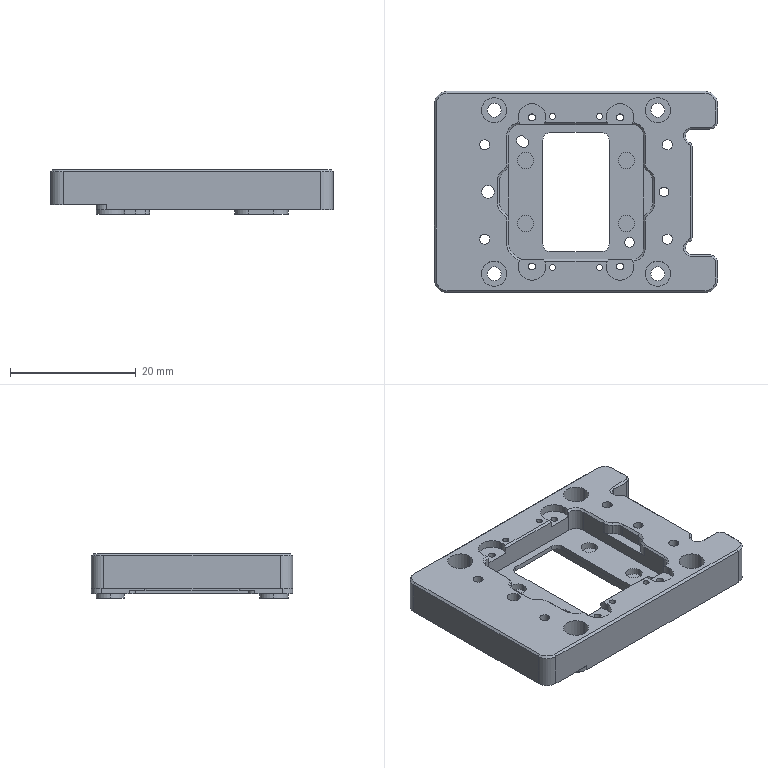NC program | NX | posted with a generic post | part box 45 x 32 x 7.05 mm
Lines 1 to 1283 of 5787:
N10 G17 G21 G94 G90
(FLOOR_WALL , TOOL : D63)
N12 T03 M6
N14 G54
N16 G17 G0 G90 X-60. Y0. S6500 M3
N18 G43 Z30. H3
N20 Z3.
N22 G94 G1 Z0. F1250.
N24 X-57.
N26 X57.
N28 X60.
N30 Z3.
N32 G0 Z30.
N34 M5
(DRILLING , TOOL : D6A45)
N36 T01 M6
N38 G54
N40 G17 G0 G90 X13. Y-13. S5000 M3
N42 G43 Z30. H1
N44 G94 G81 G98 Z-0.6 F250. R3.
N46 X14.5 Y-7.5
N48 X14. Y0.
N50 X14.5 Y7.5
N52 X13. Y13.
N54 X3.75 Y12.
N56 X7. Y11.85
N58 X8. Y5.
N60 Y-5.
N62 X8.5 Y-8.
N64 X7. Y-11.85
N66 X3.75 Y-12.
N68 X-3.75
N70 X-7. Y-11.85
N72 X-13. Y-13.
N74 X-14.5 Y-7.5
N76 X-14. Y0.
N78 X-14.5 Y7.5
N80 X-13. Y13.
N82 X-3.75 Y12.
N84 X-7. Y11.85
N86 X-8.682 Y8.171
N88 X-8. Y5.
N90 Y-5.
N92 G80
N94 G0 X-8. Y-5. Z30.
N96 M5
(DRILLING_COPY , TOOL : 1.6ZT)
N98 T11 M6
N100 G54
N102 G17 G0 G90 X-14.5 Y-7.5 S2000 M3
N104 G43 Z30. H11
N106 G94 G83 G98 Z-7.831 F100. Q1. R3.
N108 Y7.5
N110 X14.5
N112 Y-7.5
N114 G80
N116 G0 X14.5 Y-7.5 Z30.
N118 M5
(DRILLING_COPY_COPY_1 , TOOL : 1.55ZT)
N120 T20 M6
N122 G54
N124 G17 G0 G90 X14. Y0. S2000 M3
N126 G43 Z30. H20
N128 G94 G83 G98 Z-7.816 F100. Q1. R3.
N130 G80
N132 G0 X14. Y0. Z30.
N134 M5
(DRILLING_COPY_COPY , TOOL : 2.2ZT)
N136 T12 M6
N138 G54
N140 G17 G0 G90 X-13. Y13. S1447 M3
N142 G43 Z30. H12
N144 G94 G83 G98 Z-9.211 F100. Q2. R3.
N146 X13.
N148 X-13. Y-13.
N150 X13.
N152 G80
N154 G0 X13. Y-13. Z30.
N156 M5
(DRILLING_COPY_COPY_1_COPY , TOOL : 1.1ZT)
N158 T13 M6
N160 G54
N162 G17 G0 G90 X-7. Y11.85 S2000 M3
N164 G43 Z30. H13
N166 G94 G83 G98 Z-8.88 F100. Q1. R3.
N168 X7. Z-8.18
N170 Y-11.85 Z-8.88
N172 X-7. Z-8.18
N174 G80
N176 G0 X-7. Y-11.85 Z30.
N178 M5
(DRILLING_COPY_COPY_1_COPY_COPY , TOOL : 0.95ZT)
N180 T08 M6
N182 G54
N184 G17 G0 G90 X-3.75 Y-12. S2000 M3
N186 G43 Z30. H8
N188 G94 G83 G98 Z-6.385 F100. Q1. R3.
N190 X3.75
N192 Y12.
N194 X-3.75
N196 G80
N198 G0 X-3.75 Y12. Z30.
N200 M5
(DRILLING_COPY_COPY_COPY , TOOL : 2.05ZT)
N202 T09 M6
N204 G54
N206 G17 G0 G90 X-14. Y0. S1447 M3
N208 G43 Z30. H9
N210 G94 G83 G98 Z-7.966 F100. Q2. R3.
N212 G80
N214 G0 X-14. Y0. Z30.
N216 M5
(ADAPTIVE_MILLING , TOOL : D6)
N218 T06 M6
N220 G54
N222 G17 G0 G90 X-30.144 Y0.013 S9500 M3
N224 G43 Z30. H6
N226 Z-6.05
N228 G94 G1 Z-7.05 F1000.
N230 X-29.181 Y-0.309 F3000.
N232 G3 X-28.537 Y0.013 R0.611
N234 X-28.017 Y2.598 R6.628
N236 X-27.907 Y10.397 R180.736
N238 G2 X-27.877 Y17.595 R582.127
N240 X-25.501 Y20.398 R3.935
N242 X-20.894 Y21.302 R12.338
N244 X-6.645 Y21.392 R469.492
N246 G1 X23.73
N248 X23.805 Y21.391
N250 X23.88 Y21.387
N252 X23.955 Y21.381
N254 X24.029 Y21.372
N256 G2 X26.83 Y19.101 R3.89
N258 X27.783 Y14.658 R11.526
N260 X27.892 Y5.96 R211.965
N262 G1 X27.893 Y-10.84
N264 Y-17.215
N266 X27.892 Y-17.29
N268 X27.888 Y-17.365
N270 X27.882 Y-17.44
N272 X27.874 Y-17.514
N274 G2 X25.548 Y-20.356 R3.894
N276 X21.1 Y-21.289 R11.787
N278 X12.326 Y-21.392 R236.71
N280 G1 X-7.774
N282 X-23.749
N284 X-23.824 Y-21.39
N286 X-23.898 Y-21.385
N288 X-23.973 Y-21.378
N290 X-24.048 Y-21.369
N292 G2 X-26.837 Y-19.085 R3.894
N294 X-27.791 Y-14.566 R11.72
N296 X-27.862 Y-1.518 R292.418
N298 G3 X-27.319 Y9.034 R76.109
N300 G1 X-27.315 Y10.909
N302 X-27.313 Y14.509
N304 X-27.312 Y15.334
N306 X-27.31 Y15.484
N308 X-27.304 Y15.634
N310 X-27.299 Y15.709
N312 X-27.293 Y15.783
N314 X-27.285 Y15.858
N316 G2 X-24.388 Y19.606 R4.858
N318 X-19.582 Y20.651 R12.957
N320 X-10.059 Y20.785 R192.646
N322 G1 X0.441 Y20.786
N324 X21.891
N326 X21.966 Y20.785
N328 X22.116 Y20.779
N330 X22.266 Y20.768
N332 X22.34 Y20.761
N334 G2 X26.128 Y17.807 R4.868
N336 X27.158 Y12.92 R13.32
N338 X27.286 Y2.872 R220.339
N340 G1 X27.287 Y-15.353
N342 X27.286 Y-15.428
N344 X27.281 Y-15.578
N346 X27.277 Y-15.653
N348 X27.265 Y-15.802
N350 G2 X24.342 Y-19.612 R4.852
N352 X19.609 Y-20.648 R12.909
N354 X10.461 Y-20.785 R179.38
N356 G1 X3.186 Y-20.786
N358 X-21.864
N360 X-21.939 Y-20.785
N362 X-22.089 Y-20.78
N364 X-22.164 Y-20.776
N366 X-22.238 Y-20.77
N368 G2 X-26.05 Y-17.965 R4.808
N370 X-27.133 Y-13.321 R12.38
N372 X-27.224 Y-1.925 R144.317
N374 G3 X-26.723 Y11.259 R125.514
N376 G2 X-26.639 Y14.855 R31.892
N378 X-23.197 Y19.001 R5.585
N380 X-17.781 Y20.06 R15.398
N382 X-3.983 Y20.179 R359.36
N384 G1 X20.242 Y20.18
N386 X20.467 Y20.177
N388 X20.617 Y20.173
N390 X20.767 Y20.166
N392 X20.917 Y20.155
N394 G2 X25.375 Y16.923 R5.45
N396 X26.519 Y11.833 R13.725
N398 X26.68 Y0.136 R210.087
N400 X26.65 Y-14.488 R846.011
N402 X23.36 Y-18.908 R5.483
N404 X18.263 Y-20.029 R13.969
N406 X6.941 Y-20.179 R219.596
N408 G1 X-20.284 Y-20.18
N410 X-20.434 Y-20.178
N412 X-20.584 Y-20.173
N414 X-20.734 Y-20.167
N416 X-20.884 Y-20.158
N418 G2 X-25.395 Y-16.886 R5.465
N420 X-26.524 Y-11.792 R13.908
N422 X-26.331 Y1.845 R95.989
N424 G3 X-26.106 Y13.016 R282.676
N426 G2 X-25.261 Y15.849 R5.931
N428 G1 X-24.976 Y16.536
N430 X-24.935 Y16.608
N432 G2 X-21.872 Y18.959 R5.526
N434 X-12.437 Y19.556 R60.192
N436 G1 X-11.162 Y19.563
N438 X-9.587 Y19.568
N440 X-6.962 Y19.572
N442 X0.163 Y19.573
N444 X18.913
N446 X19.138 Y19.57
N448 G2 X22.118 Y18.856 R6.157
N450 X24.167 Y17.608 R5.477
N452 X25.48 Y15.291 R5.884
N454 X26.057 Y5.712 R64.333
N456 X26.042 Y-13.263 R971.054
N458 X25.356 Y-15.62 R5.962
N460 X24.108 Y-17.667 R5.475
N462 X21.791 Y-18.98 R5.884
N464 X12.812 Y-19.552 R60.138
N466 G1 X11.612 Y-19.561
N468 X10.262 Y-19.567
N470 X8.162 Y-19.571
N472 X4.037 Y-19.573
N474 X-18.913
N476 X-19.138 Y-19.57
N478 G2 X-22.102 Y-18.863 R6.151
N480 X-24.167 Y-17.608 R5.5
N482 X-25.48 Y-15.291 R5.884
N484 X-26.057 Y-4.811 R68.436
N486 X-25.65 Y3.933 R579.316
N488 G1 Y13.979
N490 X-25.647 Y14.021
N492 X-25.48 Y15.291
N494 X-25.459 Y15.372
N496 X-25.258 Y15.857
N498 X-25.104 Y16.236
N500 X-24.935 Y16.608
N502 X-24.531 Y17.145
N504 X-24.108 Y17.667
N506 X-23.58 Y18.081
N508 X-23.036 Y18.476
N510 X-22.418 Y18.739
N512 X-21.791 Y18.98
N514 X-20.521 Y19.147
N516 X-20.479 Y19.15
N518 X20.479
N520 X20.521 Y19.147
N522 X21.791 Y18.98
N524 X21.872 Y18.959
N526 X22.149 Y18.844
N528 X22.632 Y18.648
N530 X23.108 Y18.435
N532 X23.645 Y18.031
N534 X24.167 Y17.608
N536 X24.581 Y17.08
N538 X24.976 Y16.536
N540 X25.239 Y15.918
N542 X25.48 Y15.291
N544 X25.647 Y14.021
N546 G2 X25.506 Y9.626 R31.752
N548 G3 X25.475 Y-7.999 R986.646
N550 X25.65 Y-11.235 R14.601
N552 G1 Y-13.979
N554 X25.647 Y-14.021
N556 X25.48 Y-15.291
N558 X25.459 Y-15.372
N560 X25.344 Y-15.649
N562 G3 X26.613 Y-15.908 R-0.66
N564 G1 X26.673 Y-10.299
N566 X26.685 Y-9.099 Z-6.95
N568 X26.882 Y9.539
N570 X26.893 Y10.119 Z-6.998
N572 X26.882 Y10.699 Z-7.047
N574 X26.876 Y10.738 Z-7.05
N576 G3 X25.579 Y10.673 R0.66
N578 G2 X25.263 Y9.468 R4.401
N580 G3 X24.902 Y4.991 R21.417
N582 X24.901 Y-8.806 R734.54
N584 G2 X25.493 Y-10.102 R12.879
N586 G3 X26.492 Y-10.382 R0.662
N588 X26.762 Y-9.73 Z-6.988 R0.714
N590 G1 X26.759 Y-9.269 Z-6.95
N592 X26.651 Y8.966
N594 X26.653 Y9.344 Z-6.982
N596 X26.628 Y9.722 Z-7.013
N598 G3 X26.397 Y10.089 Z-7.05 R0.681
N600 X25.378 Y9.824 R0.662
N602 X24.398 Y5.67 R9.407
N604 X24.314 Y-7.902 R264.987
N606 X24.447 Y-8.296 R2.309
N608 G1 X24.995 Y-9.01
N610 G3 X25.841 Y-9.185 R0.664
N612 X26.179 Y-8.5 Z-6.983 R0.702
N614 G1 X26.181 Y-8.109 Z-6.95
N616 X26.25 Y8.181
N618 X26.254 Y8.514 Z-6.978
N620 X26.235 Y8.846 Z-7.006
N622 G3 X25.934 Y9.269 Z-7.05 R0.668
N624 X25.069 Y9.106 R0.664
N626 X24.024 Y6.498 R4.897
N628 X23.705 Y0.287 R46.885
N630 X23.734 Y-7.137 R135.875
N632 X24.237 Y-8.082 R1.07
N634 G1 X24.42 Y-8.265
N636 X24.447 Y-8.296
N638 G3 X25.255 Y-8.443 R0.665
N640 X25.606 Y-7.765 Z-6.983 R0.702
N642 G1 X25.615 Y-7.374 Z-6.95
N644 X25.966 Y7.805
N646 X25.976 Y8.14 Z-6.978
N648 X25.964 Y8.475 Z-7.006
N650 G3 X25.676 Y8.902 Z-7.05 R0.669
N652 X24.795 Y8.749 R0.664
N654 X23.442 Y5.545 R5.61
N656 X23.104 Y-1.942 R58.845
N658 X23.189 Y-6.737 R41.313
N660 X23.504 Y-7.532 R1.423
N662 G1 X24.046 Y-7.935
N664 G3 X24.782 Y-7.971 R0.666
N666 X25.103 Y-7.317 Z-6.986 R0.705
N668 G1 X25.116 Y-6.883 Z-6.95
N670 X25.53 Y7.243
N672 X25.543 Y7.582 Z-6.978
N674 X25.533 Y7.92 Z-7.007
N676 G3 X25.256 Y8.345 Z-7.05 R0.669
N678 X24.42 Y8.265 R0.664
N680 X23.087 Y5.889 R4.03
N682 X22.546 Y-0.15 R29.605
N684 X22.589 Y-5.997 R56.614
N686 X22.978 Y-7.19 R2.15
N688 G1 X23.035 Y-7.238
N690 X23.097 Y-7.279
N692 X23.16 Y-7.313
N694 X23.213 Y-7.332
N696 X23.294 Y-7.376
N698 X23.534 Y-7.555
N700 G3 X24.263 Y-7.594 R0.666
N702 X24.593 Y-6.945 Z-6.986 R0.705
N704 G1 X24.611 Y-6.512 Z-6.95
N706 X25.172 Y6.896
N708 X25.191 Y7.253 Z-6.98
N710 X25.18 Y7.61 Z-7.01
N712 G3 X24.927 Y8.009 Z-7.05 R0.673
N714 X24.142 Y8.007 R0.665
N716 X22.67 Y5.819 R3.608
N718 X22.003 Y0.626 R21.542
N720 X22.011 Y-5.445 R50.698
N722 X22.558 Y-7.05 R2.776
N724 X23.201 Y-7.328 R4.959
N726 X23.803 Y-7.25 R0.672
N728 X24.093 Y-6.621 Z-6.99 R0.719
N730 G1 X24.116 Y-6.146 Z-6.95
N732 X24.747 Y6.579
N734 X24.769 Y6.935 Z-6.98
N736 X24.76 Y7.292 Z-7.01
N738 G3 X24.509 Y7.693 Z-7.05 R0.673
N740 X23.72 Y7.693 R0.665
N742 X22.14 Y5.393 R3.832
N744 X21.65 Y3.012 R17.062
N746 X21.679 Y-5.687 R384.037
N748 X22.163 Y-6.917 R1.951
N750 G1 X22.225 Y-6.96
N752 X22.291 Y-6.996
N754 X22.714 Y-7.15
N756 G3 X23.526 Y-6.226 R0.661
N758 G1 X22.842 Y-4.922
N760 G3 X21.65 Y-5.313 R0.66
N762 X21.723 Y-6.54 R4.354
N764 X22.328 Y-7.009 R0.932
N766 X23.027 Y-5.929 R0.66
N768 G1 X22.835 Y-5.727
N770 X22.617 Y-5.554
N772 G3 X21.65 Y-6.138 R0.661
N774 X21.746 Y-6.58 R2.208
N776 X22.978 Y-6.321 R0.66
N778 G1 X23.031 Y-5.783
N780 X23.148 Y-4.589 Z-6.95
N782 X24.209 Y6.17
N784 X24.249 Y6.529 Z-6.98
N786 X24.258 Y6.889 Z-7.01
N788 G3 X24.034 Y7.298 Z-7.05 R0.674
N790 X23.294 Y7.376 R0.666
N792 X21.923 Y5.83 R2.8
N794 G1 X21.862 Y5.693
N796 X21.832 Y5.625
N798 X21.776 Y5.486
N800 X21.722 Y5.346
N802 X21.697 Y5.275
N804 X21.673 Y5.204
N806 X21.657 Y5.131
N808 X21.65 Y5.082
N810 Y2.982
N812 G3 X22.945 Y2.8 R0.66
N814 G1 X24.024 Y6.606
N816 G3 X23.143 Y7.306 R0.661
N818 X21.65 Y5.86 R2.144
N820 G1 Y5.035
N822 G3 X22.909 Y4.757 R0.66
N824 G1 X23.651 Y6.377
N826 G3 X22.79 Y7.178 R0.661
N828 X21.678 Y6.37 R1.576
N830 G1 X21.662 Y6.31
N832 X21.65 Y6.239
N834 Y5.789
N836 G3 X22.888 Y5.47 R0.66
N838 G1 X23.285 Y6.207
N840 G3 X22.438 Y7.049 R0.661
N842 X21.661 Y6.305 R0.915
N844 X21.913 Y5.709 R0.608
N846 G1 X22.153 Y5.544
N848 X23.142 Y4.864 Z-6.95
N850 X23.34 Y4.727
N852 X23.504 Y4.551
N854 X23.571 Y4.396
N856 X26.679 Y-7.193
N858 G2 X27.585 Y-12.352 R36.913
N860 X27.514 Y-14.212 R9.083
N862 G1 X27.249 Y-15.968
N864 G2 X26.238 Y-18.01 R4.668
N866 X24.779 Y-19.411 R8.489
N868 X22.342 Y-21.105 R32.788
N870 X21.529 Y-20.748 R0.602
N872 G1 X21.465 Y-20.558
N874 X21.283 Y-20.005 Z-6.999
N876 X21.085 Y-19.458 Z-7.047
N878 X21.068 Y-19.427 Z-7.05
N880 G3 X20.521 Y-19.147 R0.609
N882 G1 X20.479 Y-19.15
N884 X-20.479
N886 X-20.521 Y-19.147
N888 X-21.791 Y-18.98
N890 X-21.872 Y-18.959
N892 X-22.149 Y-18.844
N894 X-22.632 Y-18.648
N896 X-23.108 Y-18.435
N898 X-23.645 Y-18.031
N900 X-24.167 Y-17.608
N902 X-24.581 Y-17.08
N904 X-24.976 Y-16.536
N906 X-25.239 Y-15.918
N908 X-25.48 Y-15.291
N910 X-25.647 Y-14.021
N912 X-25.65 Y-13.979
N914 Y3.946
N916 G3 X-26.162 Y4.545 R0.61
N918 G1 X-27.089 Y4.69
N920 Z-4.05
N922 G0 Z30.
N924 X1.995 Y-4.659
N926 Z1.
N928 G3 X1.995 Y-4.659 Z0.821 I-1.996 J0.409 F1000.
N930 X1.995 Y-4.659 Z0.642 I-1.996 J0.409
N932 X1.995 Y-4.659 Z0.464 I-1.996 J0.409
N934 X1.995 Y-4.659 Z0.285 I-1.996 J0.409
N936 X1.995 Y-4.659 Z0.106 I-1.996 J0.409
N938 X1.995 Y-4.659 Z-0.073 I-1.996 J0.409
N940 X1.995 Y-4.659 Z-0.251 I-1.996 J0.409
N942 X1.995 Y-4.659 Z-0.43 I-1.996 J0.409
N944 X1.995 Y-4.659 Z-0.609 I-1.996 J0.409
N946 X1.995 Y-4.659 Z-0.788 I-1.996 J0.409
N948 X1.995 Y-4.659 Z-0.966 I-1.996 J0.409
N950 X1.995 Y-4.659 Z-1.145 I-1.996 J0.409
N952 X1.995 Y-4.659 Z-1.324 I-1.996 J0.409
N954 X1.995 Y-4.659 Z-1.503 I-1.996 J0.409
N956 X1.995 Y-4.659 Z-1.681 I-1.996 J0.409
N958 X1.995 Y-4.659 Z-1.86 I-1.996 J0.409
N960 X1.995 Y-4.659 Z-2.039 I-1.996 J0.409
N962 X1.995 Y-4.659 Z-2.218 I-1.996 J0.409
N964 X1.995 Y-4.659 Z-2.396 I-1.996 J0.409
N966 X1.995 Y-4.659 Z-2.575 I-1.996 J0.409
N968 X1.995 Y-4.659 Z-2.754 I-1.996 J0.409
N970 X1.995 Y-4.659 Z-2.933 I-1.996 J0.409
N972 X1.995 Y-4.659 Z-3.112 I-1.996 J0.409
N974 X1.995 Y-4.659 Z-3.29 I-1.996 J0.409
N976 X1.995 Y-4.659 Z-3.469 I-1.996 J0.409
N978 X1.995 Y-4.659 Z-3.648 I-1.996 J0.409
N980 X1.995 Y-4.659 Z-3.827 I-1.996 J0.409
N982 X1.995 Y-4.659 Z-4.005 I-1.996 J0.409
N984 X1.995 Y-4.659 Z-4.184 I-1.996 J0.409
N986 X1.995 Y-4.659 Z-4.363 I-1.996 J0.409
N988 X1.995 Y-4.659 Z-4.542 I-1.996 J0.409
N990 X1.995 Y-4.659 Z-4.72 I-1.996 J0.409
N992 X1.995 Y-4.659 Z-4.899 I-1.996 J0.409
N994 X1.995 Y-4.659 Z-5.078 I-1.996 J0.409
N996 X1.995 Y-4.659 Z-5.257 I-1.996 J0.409
N998 X1.995 Y-4.659 Z-5.435 I-1.996 J0.409
N1000 X1.995 Y-4.659 Z-5.614 I-1.996 J0.409
N1002 X1.995 Y-4.659 Z-5.793 I-1.996 J0.409
N1004 X1.995 Y-4.659 Z-5.972 I-1.996 J0.409
N1006 X1.995 Y-4.659 Z-6.15 I-1.996 J0.409
N1008 X1.995 Y-4.659 Z-6.329 I-1.996 J0.409
N1010 X1.995 Y-4.659 Z-6.508 I-1.996 J0.409
N1012 X1.995 Y-4.659 Z-6.687 I-1.996 J0.409
N1014 X1.995 Y-4.659 Z-6.865 I-1.996 J0.409
N1016 X1.995 Y-4.659 Z-7.044 I-1.996 J0.409
N1018 X2.036 Y-4.25 Z-7.05 R2.038
N1020 G1 X1.998
N1022 G3 X1.991 Y-4.411 R-1.998 F3000.
N1024 X1.872 Y-3.968 R0.835
N1026 X0.697 Y-4.157 R0.661
N1028 G1 X0.619 Y-4.412
N1030 X0.581 Y-4.676
N1032 G3 X1.829 Y-4.946 R0.66
N1034 X2.049 Y-3.516 R1.633
N1036 X-2.1 Y-3.513 R2.175
N1038 X-1.999 Y-5.151 R5.352
N1040 X-0.712 Y-6.35 R1.934
N1042 X0.925 Y-6.241 R5.105
N1044 X2.1 Y-5.02 R1.877
N1046 G1 Y-3.886
N1048 G3 X0.33 Y-1.763 R1.938
N1050 X-2.058 Y-2.833 R2.365
N1052 X-2.1 Y-3.535 R4.622
N1054 X-1.417 Y-4.195 R0.663
N1056 G1 X1.563 Y-4.085
N1058 G3 X2.1 Y-3.436 R0.664
N1060 X0.676 Y-1.574 R1.806
N1062 X-2.03 Y-2.371 R2.477
N1064 X-2.1 Y-3.065 R1.933
N1066 X-1.456 Y-3.725 R0.663
N1068 G1 X1.529 Y-3.79
N1070 G3 X2.1 Y-3.136 R0.664
N1072 X0.798 Y-1.342 R1.752
N1074 X-1.979 Y-1.924 R2.61
N1076 X-2.1 Y-2.634 R1.239
N1078 X-1.486 Y-3.293 R0.663
N1080 G1 X0.007 Y-3.402
N1082 X1.502 Y-3.493
N1084 G3 X2.1 Y-2.836 R0.664
N1086 X0.915 Y-1.112 R1.714
N1088 X-1.957 Y-1.556 R2.647
N1090 X-2.1 Y-2.29 R1.144
N1092 X-1.496 Y-2.947 R0.664
N1094 G1 X-0.003 Y-3.081
N1096 X1.493 Y-3.194
N1098 G3 X2.1 Y-2.536 R0.664
N1100 X0.961 Y-0.856 R1.701
N1102 X-1.929 Y-1.194 R2.676
N1104 X-2.1 Y-1.968 R1.076
N1106 X-1.501 Y-2.625 R0.664
N1108 G1 X-0.007 Y-2.77
N1110 X1.488 Y-2.895
N1112 G3 X2.1 Y-2.236 R0.664
N1114 X1.011 Y-0.597 R1.7
N1116 X-1.944 Y-0.888 R2.636
N1118 X-2.1 Y-1.64 R1.105
N1120 X-1.508 Y-2.297 R0.664
N1122 G1 X1.473 Y-2.596
N1124 G3 X2.1 Y-1.936 R0.663
N1126 X0.995 Y-0.302 R1.726
N1128 X-1.905 Y-0.529 R2.672
N1130 X-2.1 Y-1.321 R1.02
N1132 X-1.529 Y-1.975 R0.664
N1134 G1 X1.453 Y-2.371
N1136 G3 X2.1 Y-1.711 R0.663
N1138 X0.983 Y-0.004 R1.767
N1140 X-1.914 Y-0.227 R2.644
N1142 X-2.1 Y-1.011 R1.037
N1144 X-1.531 Y-1.664 R0.664
N1146 G1 X1.451 Y-2.071
N1148 G3 X2.1 Y-1.411 R0.663
N1150 X1.043 Y0.259 R1.754
N1152 X-1.919 Y0.078 R2.628
N1154 X-2.1 Y-0.702 R1.046
N1156 X-1.533 Y-1.355 R0.664
N1158 G1 X1.45 Y-1.771
N1160 G3 X2.1 Y-1.111 R0.663
N1162 X0.971 Y0.594 R1.797
N1164 X-1.923 Y0.383 R2.603
N1166 X-2.1 Y-0.397 R1.061
N1168 X-1.534 Y-1.05 R0.664
N1170 G1 X1.449 Y-1.471
N1172 G3 X2.1 Y-0.811 R0.663
N1174 X0.967 Y0.894 R1.813
N1176 X-1.926 Y0.687 R2.597
N1178 X-2.1 Y-0.092 R1.072
N1180 X-1.552 Y-0.743 R0.664
N1182 G1 X1.432 Y-1.246
N1184 G3 X2.1 Y-0.586 R0.663
N1186 X0.966 Y1.194 R1.832
N1188 X-1.873 Y1.044 R2.644
N1190 X-2.1 Y0.213 R0.984
N1192 X-1.553 Y-0.437 R0.664
N1194 G1 X1.431 Y-0.946
N1196 G3 X2.1 Y-0.286 R0.663
N1198 X0.964 Y1.494 R1.836
N1200 X-1.873 Y1.349 R2.633
N1202 X-2.1 Y0.518 R0.985
N1204 X-1.554 Y-0.132 R0.664
N1206 G1 X1.43 Y-0.646
N1208 G3 X2.1 Y0.014 R0.663
N1210 X0.896 Y1.828 R1.864
N1212 X-1.927 Y1.601 R2.558
N1214 X-2.1 Y0.823 R1.073
N1216 X-1.555 Y0.173 R0.664
N1218 G1 X1.429 Y-0.346
N1220 G3 X2.1 Y0.314 R0.663
N1222 X0.963 Y2.095 R1.846
N1224 X-1.873 Y1.957 R2.623
N1226 X-2.1 Y1.126 R0.984
N1228 X-1.556 Y0.477 R0.664
N1230 G1 X1.429 Y-0.046
N1232 G3 X2.1 Y0.614 R0.663
N1234 X0.963 Y2.395 R1.846
N1236 X-1.874 Y2.26 R2.631
N1238 X-2.1 Y1.431 R0.985
N1240 X-1.557 Y0.781 R0.664
N1242 G1 X1.428 Y0.254
N1244 G3 X2.1 Y0.914 R0.663
N1246 X0.963 Y2.695 R1.848
N1248 X-1.874 Y2.564 R2.626
N1250 X-2.1 Y1.735 R0.985
N1252 X-1.557 Y1.085 R0.664
N1254 G1 X1.427 Y0.554
N1256 G3 X2.1 Y1.214 R0.663
N1258 X0.963 Y2.996 R1.849
N1260 X-1.874 Y2.867 R2.626
N1262 X-2.1 Y2.038 R0.985
N1264 X-1.558 Y1.389 R0.664
N1266 G1 X1.426 Y0.854
N1268 G3 X2.1 Y1.514 R0.663
N1270 X0.963 Y3.296 R1.85
N1272 X-1.873 Y3.171 R2.624
N1274 X-2.1 Y2.341 R0.984
N1276 X-1.559 Y1.691 R0.664
N1278 G1 X1.426 Y1.154
N1280 G3 X2.1 Y1.814 R0.663
N1282 X0.964 Y3.597 R1.855
N1284 X-1.873 Y3.474 R2.625
N1286 X-2.1 Y2.644 R0.984
N1288 X-1.56 Y1.995 R0.664
N1290 G1 X1.425 Y1.454
N1292 G3 X2.1 Y2.114 R0.663
N1294 X0.964 Y3.897 R1.854
N1296 X-1.873 Y3.776 R2.621
N1298 X-2.1 Y2.945 R0.984
N1300 X-1.56 Y2.296 R0.664
N1302 G1 X1.425 Y1.754
N1304 G3 X2.1 Y2.414 R0.663
N1306 X1.03 Y4.162 R1.831
N1308 X-1.872 Y4.079 R2.63
N1310 X-2.1 Y3.247 R0.983
N1312 X-1.56 Y2.598 R0.664
N1314 G1 X1.424 Y2.054
N1316 G3 X2.1 Y2.714 R0.663
N1318 X0.966 Y4.499 R1.857
N1320 X-1.924 Y4.331 R2.556
N1322 X-2.1 Y3.55 R1.067
N1324 X-1.561 Y2.901 R0.664
N1326 G1 X1.424 Y2.354
N1328 G3 X2.1 Y3.014 R0.663
N1330 X0.968 Y4.8 R1.86
N1332 X-1.869 Y4.686 R2.618
N1334 X-2.1 Y3.854 R0.977
N1336 X-1.562 Y3.205 R0.664
N1338 G1 X1.423 Y2.654
N1340 G3 X2.1 Y3.314 R0.663
N1342 X0.968 Y5.101 R1.862
N1344 X-1.869 Y4.99 R2.619
N1346 X-2.1 Y4.158 R0.976
N1348 X-1.563 Y3.509 R0.664
N1350 G1 X1.422 Y2.954
N1352 G3 X2.1 Y3.614 R0.663
N1354 X0.969 Y5.402 R1.865
N1356 X-1.868 Y5.294 R2.619
N1358 X-2.1 Y4.462 R0.973
N1360 X-1.563 Y3.814 R0.664
N1362 G1 X1.421 Y3.254
N1364 G3 X2.1 Y3.914 R0.663
N1366 X0.97 Y5.702 R1.864
N1368 X-1.866 Y5.596 R2.613
N1370 X-2.1 Y4.765 R0.971
N1372 X-1.564 Y4.117 R0.664
N1374 G1 X1.421 Y3.554
N1376 G3 X2.1 Y4.214 R0.663
N1378 X0.972 Y6.004 R1.872
N1380 X-1.878 Y5.887 R2.615
N1382 X-2.1 Y5.137 R0.895
N1384 X-1.58 Y4.492 R0.664
N1386 G1 X-0.088 Y4.165
N1388 X1.406 Y3.855
N1390 G3 X2.1 Y4.514 R0.663
N1392 X0.773 Y6.35 R1.802
N1394 G1 X-0.202
N1396 G3 X-0.512 Y5.108 R0.66
N1398 G1 X1.225 Y4.19
N1400 G3 X2.1 Y4.814 R0.662
N1402 X1.249 Y6.335 R1.414
N1404 G1 X1.163 Y6.35
N1406 X0.713
N1408 G3 X0.303 Y5.173 R0.661
N1410 G1 X1.118 Y4.538
N1412 G3 X2.1 Y5.114 R0.661
N1414 X1.616 Y6.289 R1.151
N1416 X1.148 Y6.35 R2.349
N1418 X0.694 Y5.211 R0.661
N1420 G1 X1.072 Y4.866
N1422 G3 X2.1 Y5.414 R0.661
N1424 X1.423 Y6.345 R0.78
N1426 G1 X-0.559 Y6.35
N1428 G3 X-1.859 Y6.114 R2.034
N1430 X-2.1 Y5.398 R0.828
N1432 X-0.964 Y4.941 R0.661
N1434 G1 X-0.75 Y5.157
N1436 X-0.566 Y5.4
N1438 G3 X-1.159 Y6.35 R0.661
N1440 X-2.095 Y5.673 R0.782
N1442 X-1.656 Y5.036 R0.604
N1444 G1 X-1.367 Y5.011 Z-7.026
N1446 X-1.076 Z-7.001
N1448 G2 X-0.586 Y4.682 Z-6.95 R0.603
N1450 G1 X-0.544 Y4.551
N1452 X-0.523 Y4.414
N1454 X-0.531 Y-3.524
N1456 X-0.58 Y-3.689
N1458 G2 X-1.232 Y-4.038 Z-7.016 R0.637
N1460 G1 X-1.64 Y-4.055 Z-7.05
N1462 G3 X-2.1 Y-4.638 R0.605
N1464 X-1.252 Y-6.326 R1.591
N1466 G1 X-1.179 Y-6.342
N1468 X-1.125 Y-6.35
N1470 X-0.675
N1472 G3 X-0.267 Y-5.171 R0.661
N1474 G1 X-1.12 Y-4.511
N1476 G3 X-2.1 Y-5.088 R0.661
N1478 X-1.555 Y-6.306 R1.152
N1480 G1 X-1.069 Y-6.35
N1482 G3 X-0.652 Y-5.178 R0.661
N1484 G1 X-1.111 Y-4.816
N1486 G3 X-2.1 Y-5.388 R0.661
N1488 X-1.298 Y-6.35 R0.79
N1490 G1 X0.413
N1492 G3 X2.065 Y-5.559 R1.604
N1494 G1 X2.1 Y-4.951
N1496 G3 X0.945 Y-4.515 R0.661
N1498 G1 X0.229 Y-5.34
N1500 G3 X0.788 Y-6.35 R0.661
N1502 X2.003 Y-5.926 R1.313
N1504 X2.1 Y-5.398 R1.21
N1506 X0.961 Y-4.944 R0.661
N1508 G1 X0.75 Y-5.161
N1510 X0.569 Y-5.404
N1512 G3 X1.163 Y-6.35 R0.661
N1514 X2.1 Y-5.623 R0.78
N1516 X1.625 Y-5.032 R0.611
N1518 G1 X0.589 Y-4.802
N1520 Z-4.05
N1522 G0 Z30.
N1524 X-0.622 Y0.875
N1526 Z-2.699
N1528 G1 Z-3.699 F1000.
N1530 X-1.917 Y0.259 F3000.
N1532 X-2.044 Y0.144
N1534 X-2.138 Y0.
N1536 G3 X-2.658 Y-2.968 R8.162
N1538 X-2.557 Y-5.579 R8.699
N1540 X-1.093 Y-6.696 R1.694
N1542 X1.502 Y-6.713 R5.123
N1544 X2.407 Y-5.427 R1.569
N1546 X2.723 Y-0.87 R25.535
N1548 X2.685 Y5.053 R80.998
N1550 X1.184 Y6.661 R1.659
N1552 X-1.486 Y6.717 R5.369
N1554 X-2.419 Y5.369 R1.612
N1556 X-2.735 Y1.636 R27.994
N1558 X-3.227 Y-4.037 R43.398
N1560 X-2.441 Y-6.318 R3.222
N1562 X1.514 Y-7.027 R4.121
N1564 X2.787 Y-5.26 R2.599
N1566 X3.284 Y-0.724 R19.395
N1568 X3.254 Y4.448 R50.158
N1570 X1.043 Y7.039 R2.731
N1572 X-1.663 Y6.947 R3.641
N1574 X-2.832 Y5.094 R2.852
N1576 X-3.408 Y1.089 R38.498
N1578 X-3.721 Y-4.068 R26.237
N1580 X-0.637 Y-7.528 R3.633
N1582 X1.484 Y-7.35 R4.911
N1584 X3.146 Y-5.322 R3.253
N1586 X3.832 Y-0.74 R16.416
N1588 X3.772 Y4.278 R29.237
N1590 X0.684 Y7.512 R3.707
N1592 X-1.586 Y7.304 R4.474
N1594 X-3.207 Y5.144 R3.484
N1596 X-4.272 Y-3.388 R32.466
N1598 X-2.843 Y-6.825 R4.794
N1600 X-1.635 Y-7.55 R2.909
N1602 G1 X0.536
N1604 G3 X3.136 Y-6.152 R2.543
N1606 X4.264 Y-2.062 R10.109
N1608 X4.337 Y3.85 R27.376
N1610 X1.745 Y7.533 R4.484
N1612 G1 X1.671 Y7.547
N1614 X1.648 Y7.55
N1616 X0.448
N1618 G3 X-0.113 Y7.237 R0.67
N1620 X-0.201 Y6.683 Z-3.651 R0.86
N1622 G1 X-0.167 Y6.057 Z-3.599
N1624 X0.502 Y-6.031
N1626 X0.565 Y-7.027 Z-3.682
N1628 X0.636 Y-7.215 Z-3.699
N1630 G3 X1.211 Y-7.55 R0.67
N1632 X3.26 Y-6.528 R2.269
N1634 X4.695 Y-2.627 R8.503
N1636 X4.828 Y3.872 R21.837
N1638 X2.554 Y7.506 R5.136
N1640 X1.619 Y7.55 R4.681
N1642 X1.058 Y7.237 R0.67
N1644 X0.959 Y6.712 Z-3.654 R0.908
N1646 G1 X0.957 Y6.055 Z-3.599
N1648 X0.928 Y-6.033
N1650 X0.922 Y-6.525 Z-3.64
N1652 X0.94 Y-7.017 Z-3.681
N1654 X1.013 Y-7.218 Z-3.699
N1656 G3 X1.586 Y-7.55 R0.67
N1658 X3.596 Y-6.595 R2.284
N1660 X5.198 Y-2.602 R8.525
N1662 X5.303 Y3.962 R18.519
N1664 X3.275 Y7.453 R5.792
N1666 X2.308 Y7.55 R2.079
N1668 X1.746 Y7.235 R0.67
N1670 X1.643 Y6.679 Z-3.651 R1.033
N1672 G1 X1.627 Y6.054 Z-3.599
N1674 X1.322 Y-6.034
N1676 X1.305 Y-6.521 Z-3.64
N1678 X1.313 Y-7.008 Z-3.68
N1680 X1.388 Y-7.218 Z-3.699
N1682 G3 X1.961 Y-7.55 R0.67
N1684 X4.034 Y-6.555 R2.377
N1686 X5.701 Y-2.587 R8.757
N1688 X5.76 Y4.116 R16.384
N1690 X3.86 Y7.444 R6.01
N1692 X2.952 Y7.55 R1.787
N1694 X2.389 Y7.234 R0.67
N1696 X2.283 Y6.688 Z-3.652 R1.064
N1698 G1 X2.254 Y6.053 Z-3.599
N1700 X1.713 Y-6.035
N1702 X1.686 Y-6.517 Z-3.639
N1704 X1.687 Y-7. Z-3.68
N1706 X1.763 Y-7.218 Z-3.699
N1708 G3 X2.336 Y-7.55 R0.67
N1710 X4.425 Y-6.58 R2.431
N1712 X6.218 Y-2.506 R8.824
N1714 X6.177 Y4.406 R15.006
N1716 X4.443 Y7.417 R6.054
N1718 X3.495 Y7.55 R1.607
N1720 X2.932 Y7.233 R0.67
N1722 X2.824 Y6.691 Z-3.652 R1.093
N1724 G1 X2.791 Y6.052 Z-3.599
N1726 X2.169 Y-6.035
N1728 X2.138 Y-6.516 Z-3.639
N1730 X2.136 Y-6.997 Z-3.679
N1732 X2.214 Y-7.219 Z-3.699
N1734 G3 X2.786 Y-7.55 R0.67
N1736 X4.871 Y-6.558 R2.513
N1738 X6.752 Y-2.362 R9.07
N1740 X6.567 Y4.759 R14.177
N1742 X4.966 Y7.424 R5.703
N1744 X4.023 Y7.55 R1.662
N1746 X3.458 Y7.232 R0.67
N1748 X3.349 Y6.697 Z-3.653 R1.114
N1750 G1 X3.309 Y6.051 Z-3.599
N1752 X2.553 Y-6.036
N1754 X2.517 Y-6.514 Z-3.639
N1756 X2.511 Y-6.993 Z-3.679
N1758 X2.589 Y-7.219 Z-3.699
N1760 G3 X3.161 Y-7.55 R0.67
N1762 X5.268 Y-6.599 R2.552
N1764 X7.268 Y-2.298 R9.078
N1766 G1 X7.55 Y-0.466
N1768 G3 X7.364 Y3.572 R21.543
N1770 X5.67 Y7.271 R7.167
N1772 X5.15 Y7.55 R1.051
N1774 G1 X4.55
N1776 G3 X3.955 Y7.176 R0.669
N1778 X3.999 Y6.51 Z-3.641 R0.717
N1780 G1 X4.211 Y6.053 Z-3.599
N1782 X6.04 Y2.121
N1784 X6.194 Y1.781 Z-3.63
N1786 X6.372 Y1.453 Z-3.661
N1788 G3 X6.745 Y1.215 Z-3.699 R0.678
N1790 X7.55 Y1.859 R0.662
N1792 X7.447 Y4.701 R15.562
N1794 X5.985 Y7.429 R4.871
N1796 X5.125 Y7.55 R1.522
N1798 X4.555 Y6.556 R0.661
N1800 G1 X5.461 Y5.004
N1802 X6.383 Y3.461
N1804 G3 X7.55 Y3.884 R0.661
N1806 X7.292 Y6.175 R5.663
N1808 X6.267 Y7.514 R2.368
N1810 X5.581 Y7.55 R9.137
N1812 X5.039 Y6.513 R0.661
N1814 G1 X6.414 Y4.551
N1816 G3 X7.55 Y5.009 R0.661
N1818 X7.116 Y7.095 R3.318
N1820 X6.095 Y7.55 R0.97
N1822 X5.567 Y6.493 R0.661
N1824 G1 X6.431 Y5.36
N1826 G3 X7.55 Y5.834 R0.661
N1828 X7.143 Y7.379 R2.002
N1830 X6.443 Y7.55 R0.971
N1832 X5.938 Y6.465 R0.661
N1834 G1 X6.46 Y5.858
N1836 G3 X7.55 Y6.359 R0.661
N1838 X7.275 Y7.392 R1.207
N1840 X6.673 Y7.55 R1.039
N1842 X6.503 Y6.252 R0.66
N1844 X7.031 Y6.189 R1.075
N1846 X7.475 Y7.13 R0.662
N1848 X6.823 Y7.55 R0.732
N1850 G1 X-0.497
N1852 G3 X-3.116 Y6.183 R2.556
N1854 X-4.334 Y2.343 R11.441
N1856 X-4.749 Y-3.623 R22.148
N1858 X-2.587 Y-7.482 R5.142
N1860 X-1.598 Y-7.55 R2.875
N1862 X-1.036 Y-7.236 R0.67
N1864 X-0.931 Y-6.682 Z-3.651 R1.04
N1866 G1 X-0.912 Y-6.054 Z-3.599
N1868 X-0.538 Y6.033
N1870 X-0.517 Y6.519 Z-3.64
N1872 X-0.523 Y7.005 Z-3.68
N1874 X-0.599 Y7.218 Z-3.699
N1876 G3 X-1.172 Y7.55 R0.67
N1878 X-3.234 Y6.554 R2.279
N1880 X-4.77 Y2.763 R9.305
N1882 X-5.236 Y-3.64 R19.12
N1884 X-3.231 Y-7.459 R5.67
N1886 X-2.347 Y-7.55 R1.954
N1888 X-1.783 Y-7.234 R0.67
N1890 X-1.675 Y-6.692 Z-3.652 R1.093
N1892 G1 X-1.642 Y-6.053 Z-3.599
N1894 X-1.006 Y6.034
N1896 X-0.975 Y6.515 Z-3.639
N1898 X-0.972 Y6.996 Z-3.679
N1900 X-1.049 Y7.218 Z-3.699
N1902 G3 X-1.622 Y7.55 R0.67
N1904 X-3.619 Y6.563 R2.316
N1906 X-5.323 Y2.603 R9.559
N1908 X-5.699 Y-3.797 R16.831
N1910 X-3.863 Y-7.402 R6.062
N1912 X-2.898 Y-7.55 R1.531
N1914 X-2.334 Y-7.233 R0.67
N1916 X-2.224 Y-6.698 Z-3.653 R1.117
N1918 G1 X-2.182 Y-6.052 Z-3.599
N1920 X-1.391 Y6.035
N1922 X-1.354 Y6.512 Z-3.639
N1924 X-1.346 Y6.991 Z-3.679
N1926 X-1.424 Y7.218 Z-3.699
N1928 G3 X-1.997 Y7.55 R0.67
N1930 X-4.01 Y6.584 R2.391
N1932 X-5.873 Y2.453 R9.603
N1934 X-6.095 Y-4.236 R14.955
N1936 X-4.435 Y-7.37 R6.045
N1938 X-4.028 Y-7.55 R1.403
N1940 G1 X-3.428
N1942 G3 X-2.863 Y-7.232 R0.67
N1944 X-2.751 Y-6.703 Z-3.654 R1.141
N1946 G1 X-2.701 Y-6.052 Z-3.599
N1948 X-1.775 Y6.035
N1950 X-1.733 Y6.51 Z-3.639
N1952 X-1.721 Y6.986 Z-3.679
N1954 X-1.799 Y7.218 Z-3.699
N1956 G3 X-2.372 Y7.55 R0.67
N1958 X-4.456 Y6.561 R2.486
N1960 X-6.403 Y2.388 R9.697
N1962 X-6.474 Y-4.661 R14.037
N1964 X-4.892 Y-7.419 R5.556
N1966 X-4.02 Y-7.55 R1.466
N1968 X-3.455 Y-7.23 R0.67
N1970 G1 X-3.369 Y-6.984 Z-3.677
N1972 X-3.342 Y-6.726 Z-3.656
N1974 X-3.28 Y-6.051 Z-3.599
N1976 X-2.163 Y6.036
N1978 X-2.088 Y6.93 Z-3.674
N1980 X-2.119 Y7.077 Z-3.686
N1982 X-2.174 Y7.217 Z-3.699
N1984 G3 X-2.747 Y7.55 R0.67
N1986 X-4.907 Y6.547 R2.594
N1988 X-6.997 Y2.037 R9.947
N1990 X-6.814 Y-5.146 R13.316
N1992 X-5.349 Y-7.456 R4.822
N1994 X-4.536 Y-7.55 R1.734
N1996 X-3.97 Y-7.229 R0.67
N1998 X-3.851 Y-6.674 Z-3.651 R1.331
N2000 G1 X-3.787 Y-6.05 Z-3.599
N2002 X-2.546 Y6.037
N2004 X-2.463 Y6.925 Z-3.673
N2006 X-2.493 Y7.075 Z-3.686
N2008 X-2.549 Y7.217 Z-3.699
N2010 G3 X-3.122 Y7.55 R0.67
N2012 X-5.36 Y6.543 R2.686
N2014 X-7.55 Y1.828 R9.902
N2016 X-7.521 Y-3.871 R489.075
N2018 X-6.03 Y-7.318 R5.79
N2020 X-5.038 Y-7.55 R1.23
N2022 X-4.456 Y-6.579 R0.661
N2024 G1 X-6.308 Y-3.111
N2026 G3 X-7.55 Y-3.422 R0.66
N2028 X-7.411 Y-5.658 R8.32
N2030 X-6.287 Y-7.472 R3.291
N2032 X-5.5 Y-7.55 R1.965
N2034 X-4.949 Y-6.528 R0.661
N2036 G1 X-6.403 Y-4.326
N2038 G3 X-7.55 Y-4.772 R0.661
N2040 X-7.194 Y-6.883 R3.871
N2042 X-5.968 Y-7.55 R1.088
N2044 X-5.441 Y-6.492 R0.661
N2046 G1 X-6.437 Y-5.192
N2048 G3 X-7.55 Y-5.672 R0.661
N2050 X-7.118 Y-7.363 R2.255
N2052 X-6.409 Y-7.55 R0.935
N2054 X-5.888 Y-6.485 R0.661
N2056 G1 X-6.443 Y-5.786
N2058 G3 X-7.55 Y-6.272 R0.661
N2060 X-7.319 Y-7.339 R1.464
N2062 X-6.673 Y-7.55 R0.872
N2064 X-6.268 Y-6.369 R0.661
N2066 G1 X-6.459 Y-6.22
N2068 X-6.669 Y-6.1
N2070 G3 X-7.55 Y-6.722 R0.662
N2072 X-7.145 Y-7.467 R0.761
N2074 G1 X-6.553 Y-7.367
N2076 G3 X-6.188 Y-7.176 R0.705
N2078 X-5.979 Y-6.687 Z-3.654 R0.912
N2080 G1 X-5.834 Y-6.044 Z-3.599
N2082 X-3.127 Y5.944
N2084 X-3.015 Y6.41 Z-3.639
N2086 X-2.932 Y6.883 Z-3.679
N2088 X-2.973 Y7.118 Z-3.699
N2090 X-3.017 Y7.212
N2092 X-3.076 Y7.298
N2094 X-3.147 Y7.374
N2096 G3 X-4.096 Y7.545 R1.244
N2098 X-6.257 Y6.036 R3.55
N2100 X-7.55 Y3.532 R8.774
N2102 G1 Y1.807
N2104 G3 X-6.847 Y1.148 R0.663
N2106 X-6.262 Y1.578 Z-3.635 R0.706
N2108 G1 X-6.047 Y1.957 Z-3.599
N2110 X-3.749 Y6.03
N2112 X-3.559 Y6.359 Z-3.631
N2114 X-3.391 Y6.7 Z-3.663
N2116 G3 X-3.407 Y7.13 Z-3.699 R0.682
N2118 X-4.022 Y7.55 R0.666
N2120 X-6.274 Y6.558 R2.784
N2122 X-7.549 Y4.638 R5.055
N2124 X-6.439 Y4.155 R0.661
N2126 G1 X-3.951 Y6.485
N2128 G3 X-4.472 Y7.55 R0.661
N2130 X-6.785 Y6.519 R2.858
N2132 X-7.55 Y5.415 R2.56
N2134 G1 Y3.465
N2136 G3 X-6.318 Y3.136 R0.66
N2138 G1 X-5.303 Y4.892
N2140 X-4.304 Y6.657
N2142 G3 X-4.922 Y7.55 R0.662
N2144 X-7.525 Y6.096 R2.805
N2146 G1 X-7.542 Y6.023
N2148 X-7.55 Y6.002
N2150 Y5.402
N2152 G3 X-6.428 Y4.93 R0.661
N2154 G1 X-4.841 Y6.497
N2156 G3 X-5.372 Y7.55 R0.661
N2158 X-7.507 Y6.575 R2.183
N2160 X-7.55 Y5.943 R4.216
N2162 X-6.452 Y5.449 R0.661
N2164 G1 X-5.31 Y6.473
N2166 G3 X-5.822 Y7.55 R0.661
N2168 X-7.513 Y6.914 R1.811
N2170 G1 X-7.521 Y6.893
N2172 X-7.531 Y6.855
N2174 X-7.55 Y6.699
N2176 Y6.324
N2178 G3 X-6.444 Y5.837 R0.661
N2180 G1 X-5.754 Y6.48
N2182 G3 X-6.272 Y7.55 R0.661
N2184 X-7.513 Y6.912 R1.1
N2186 G1 X-7.374 Y6.329
N2188 X-7.323 Y6.2
N2190 X-7.255 Y6.08
N2192 X-6.767 Y5.446
N2194 X-6.035 Y4.495 Z-3.599
N2196 X2.075 Y-6.044
N2198 X2.807 Y-6.995 Z-3.699
N2200 X3.032 Y-7.288
N2202 X3.07 Y-7.333
N2204 X3.112 Y-7.374
N2206 G3 X3.986 Y-7.55 R1.16
N2208 X6.018 Y-6.256 R3.119
N2210 X7.55 Y-3.105 R8.791
N2212 G1 Y-0.405
N2214 G3 X6.756 Y0.241 R0.662
N2216 X6.241 Y-0.241 Z-3.637 R0.714
N2218 G1 X6.052 Y-0.661 Z-3.599
N2220 X3.649 Y-6.027
N2222 X3.485 Y-6.384 Z-3.632
N2224 X3.342 Y-6.751 Z-3.665
N2226 G3 X3.381 Y-7.154 Z-3.699 R0.689
N2228 X3.986 Y-7.55 R0.668
N2230 X6.225 Y-6.538 R2.717
N2232 X7.55 Y-4.386 R5.614
N2234 G1 Y-3.036
N2236 G3 X6.902 Y-2.376 R0.663
N2238 X6.271 Y-2.78 Z-3.633 R0.708
N2240 G1 X6.051 Y-3.125 Z-3.599
N2242 X4.2 Y-6.032
N2244 X3.996 Y-6.345 Z-3.63
N2246 X3.815 Y-6.671 Z-3.661
N2248 G3 X3.815 Y-7.114 Z-3.699 R0.678
N2250 X4.436 Y-7.55 R0.666
N2252 X6.68 Y-6.544 R2.76
N2254 X7.55 Y-5.298 R3.708
N2256 G1 Y-4.323
N2258 G3 X6.377 Y-3.908 R0.661
N2260 G1 X5.301 Y-5.23
N2262 X4.238 Y-6.562
N2264 G3 X4.811 Y-7.55 R0.661
N2266 X7.187 Y-6.497 R2.836
N2268 X7.55 Y-5.909 R1.479
N2270 G1 Y-5.234
N2272 G3 X6.419 Y-4.771 R0.661
N2274 G1 X4.724 Y-6.506
N2276 G3 X5.261 Y-7.55 R0.661
N2278 X7.511 Y-6.492 R2.295
N2280 X7.55 Y-5.873 R6.787
N2282 X6.459 Y-5.374 R0.661
N2284 G1 X5.205 Y-6.466
N2286 G3 X5.711 Y-7.55 R0.661
N2288 X7.464 Y-6.921 R1.942
N2290 X7.55 Y-6.263 R1.515
N2292 X6.433 Y-5.786 R0.661
N2294 G1 X5.71 Y-6.492
N2296 G3 X6.236 Y-7.55 R0.661
N2298 X7.413 Y-7.208 R1.392
N2300 G1 X7.454 Y-7.145
N2302 X7.489 Y-7.079
N2304 G3 X6.45 Y-6.479 R0.81
N2306 G1 Z-0.699
N2308 G0 Z30.
N2310 X6.3 Y-6.391
N2312 Z-2.699
N2314 G1 Z-3.699 F1000.
N2316 G3 X6.611 Y-7.55 R0.63 F3000.
N2318 X7.55 Y-6.598 R0.802
N2320 X6.913 Y-5.993 R0.609
N2322 G1 X6.039 Y-6.038
N2324 Z-0.699
N2326 G0 Z30.
N2328 X6.082 Y-4.291
N2330 Z-0.763
N2332 G1 Z-1.763 F1000.
N2334 X6.999 Y-4.49 F3000.
N2336 G3 X7.634 Y-3.962 R0.61
N2338 G2 X7.968 Y-2.267 R27.249
N2340 G3 X8.146 Y2.29 R25.885
N2342 G2 X7.624 Y4.035 R4.925
N2344 G3 X6.313 Y4.014 R0.66
N2346 G1 X6.332 Y2.814 Z-1.663
N2348 X6.435 Y-2.531
N2350 X6.438 Y-2.905 Z-1.694
N2352 X6.468 Y-3.279 Z-1.725
N2354 G3 X6.71 Y-3.647 Z-1.763 R0.679
N2356 X7.72 Y-3.362 R0.662
N2358 X8.657 Y1.476 R10.242
N2360 X8.146 Y2.29 R3.913
N2362 G1 X8.118 Y2.36
N2364 G3 X7.138 Y2.665 R0.662
N2366 X6.846 Y1.998 Z-1.699 R0.706
N2368 G1 X6.853 Y1.564 Z-1.663
N2370 X6.898 Y-1.449
N2372 X6.901 Y-1.787 Z-1.691
N2374 X6.926 Y-2.125 Z-1.719
N2376 G3 X7.222 Y-2.538 Z-1.763 R0.669
N2378 X8.146 Y-2.29 R0.663
N2380 X8.994 Y1.063 R4.487
N2382 G1 X8.926 Y1.183
N2384 X8.577 Y1.671
N2386 G3 X7.382 Y1.328 R0.661
N2388 G1 X7.207 Y-1.599
N2390 G3 X8.401 Y-1.918 R0.661
N2392 X9.038 Y-0.909 R4.279
N2394 X7.879 Y-0.598 R0.703
N2396 G1 Z1.238
N2398 G0 Z30.
N2400 X7.841 Y-0.647
N2402 Z-0.763
N2404 G1 Z-1.763 F1000.
N2406 G3 X8.88 Y-1.247 R0.607 F3000.
N2408 X9.05 Y-0.787 R1.073
N2410 G1 Y0.188
N2412 G3 X8.252 Y0.763 R0.608
N2414 G1 X7.539 Y0.525
N2416 Z1.238
N2418 G0 Z30.
N2420 X-6.083 Y4.288
N2422 Z-0.763
N2424 G1 Z-1.763 F1000.
N2426 X-6.996 Y4.49 F3000.
N2428 G3 X-7.634 Y3.962 R0.61
N2430 G2 X-7.958 Y2.341 R20.508
N2432 G3 X-8.146 Y-2.29 R25.713
N2434 G2 X-7.624 Y-4.035 R4.925
N2436 G3 X-6.313 Y-4.014 R0.66
N2438 G1 X-6.332 Y-2.814 Z-1.663
N2440 X-6.435 Y2.531
N2442 X-6.438 Y2.905 Z-1.694
N2444 X-6.468 Y3.279 Z-1.725
N2446 G3 X-6.71 Y3.647 Z-1.763 R0.679
N2448 X-7.72 Y3.362 R0.662
N2450 X-8.635 Y-1.548 R9.511
N2452 G1 X-8.606 Y-1.617
N2454 X-8.6 Y-1.639
N2456 X-8.183 Y-2.223
N2458 X-8.146 Y-2.29
N2460 X-8.118 Y-2.36
N2462 G3 X-7.138 Y-2.665 R0.662
N2464 X-6.846 Y-1.998 Z-1.699 R0.706
N2466 G1 X-6.853 Y-1.564 Z-1.663
N2468 X-6.898 Y1.449
N2470 X-6.901 Y1.788 Z-1.691
N2472 X-6.926 Y2.125 Z-1.719
N2474 G3 X-7.222 Y2.538 Z-1.763 R0.669
N2476 X-8.146 Y2.29 R0.663
N2478 X-8.994 Y-1.063 R4.479
N2480 G1 X-8.926 Y-1.183
N2482 X-8.577 Y-1.671
N2484 G3 X-7.382 Y-1.328 R0.661
N2486 G1 X-7.207 Y1.599
N2488 G3 X-8.401 Y1.918 R0.661
N2490 X-9.039 Y0.907 R4.242
N2492 G1 X-9.05 Y0.787
N2494 Y-0.188
N2496 G3 X-7.731 Y-0.217 R0.66
N2498 G1 X-7.688 Y0.939
N2500 G3 X-8.88 Y1.247 R0.661
N2502 G1 X-8.926 Y1.183
N2504 X-8.994 Y1.063
N2506 X-9.016 Y0.991
N2508 G3 X-8.475 Y0.209 R0.608
N2510 G1 X-7.541 Y0.148
N2512 Z1.238
N2514 G0 Z30.
N2516 M5